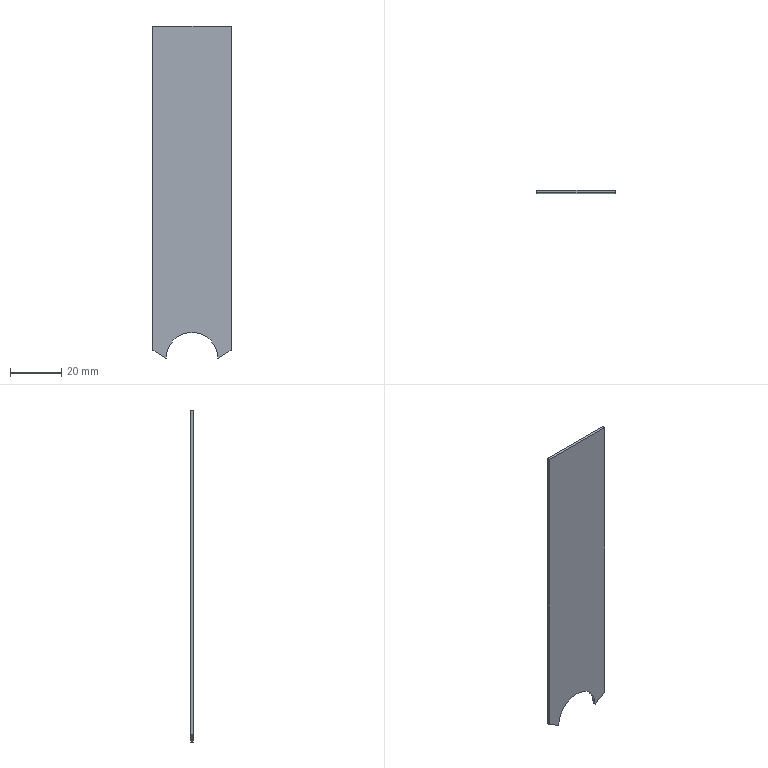Part | STEP file | solid 166 | 1 solid | 10 faces | box 30.5 x 1 x 129.425 mm | volume 3778 mm3 | plane 5 | cylinder 3 | cone 2 | commonest cylinder face diameters 30.5 x2 20 x1